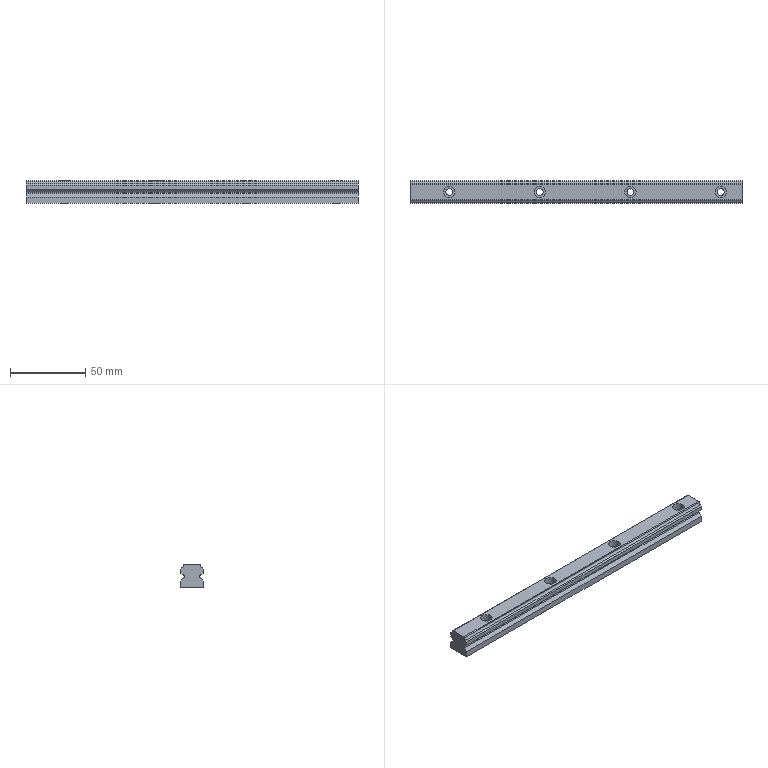Part | STEP file | Tube feed_id598_x_t | 1 solid | 34 faces | box 220 x 15 x 15 mm | volume 42972 mm3 | plane 18 | cylinder 16 | commonest cylinder face diameters 3 x6 4.5 x4 7.6 x4 1 x2